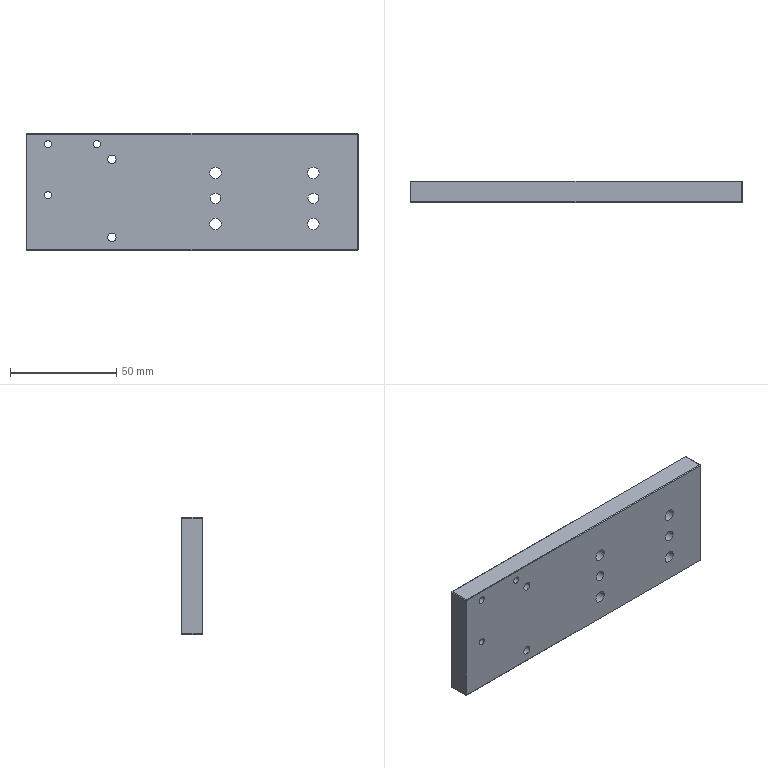Part | NX | 1 solid | 74 faces | box 156 x 10 x 55 mm | volume 82821 mm3 | cylinder 34 | plane 22 | cone 18 | commonest cylinder face diameters 5.5 x8 9.5 x8 3.3 x6 2.5 x4 4 x4 5 x4